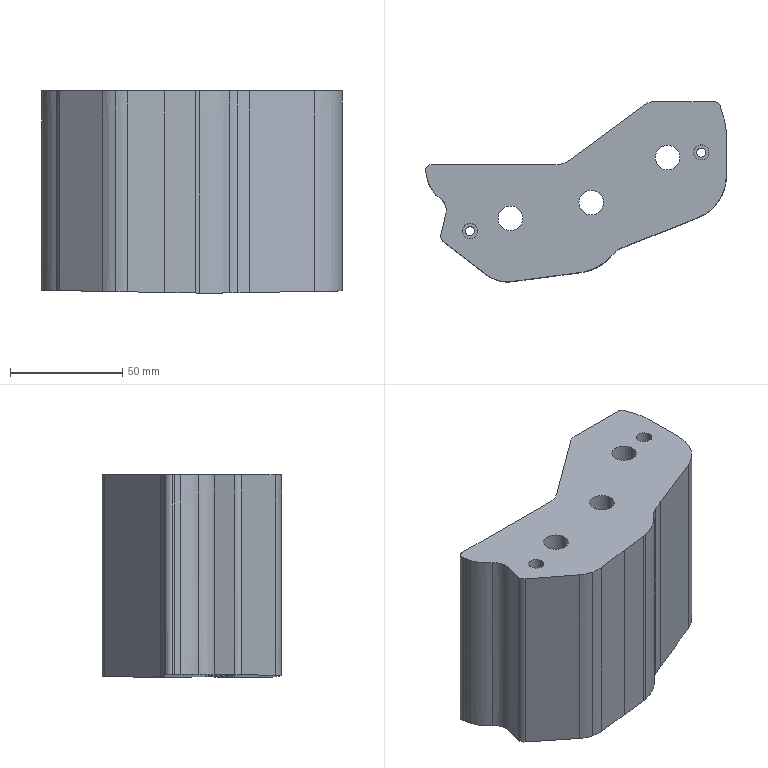Part | STEP file | gslz 2016.10.28-10_id2986_x_t | 1 solid | 49 faces | box 134.015 x 80.135 x 90 mm | volume 527779 mm3 | other 18 | cylinder 16 | plane 14 | spline 1 | commonest cylinder face diameters 5 x4 11 x3 17 x3 4.1 x2 6.8 x2 10 x1